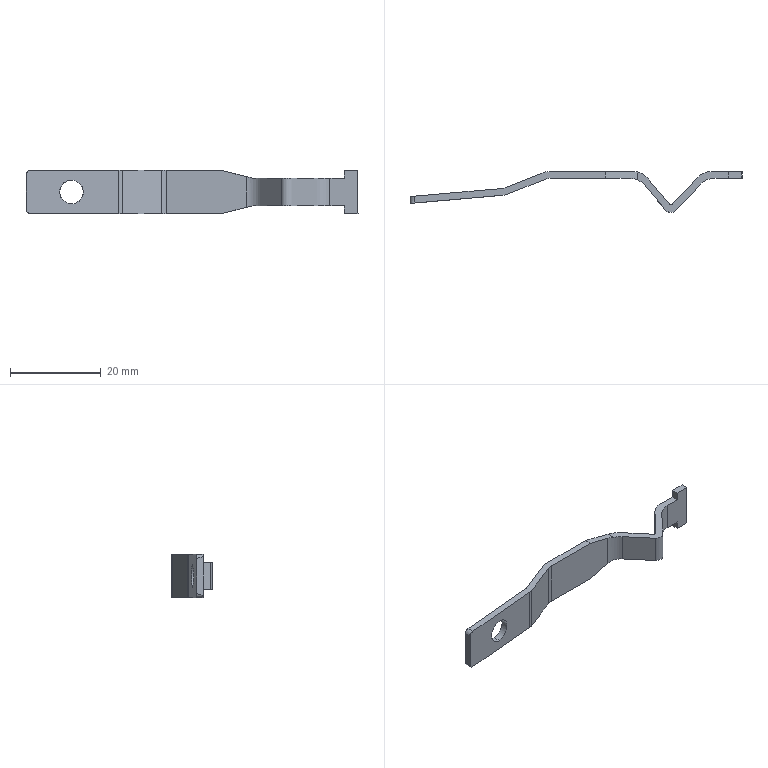Part | SolidWorks | features Extrusion 1, ICE 1 | 1 solid | 38 faces | box 73 x 9 x 9.5 mm | volume 954.396 mm3 | plane 24 | cylinder 14 | commonest cylinder face diameters 6 x4 8 x4 2 x2 5.2 x2 1 x1 3 x1
STEP:
#1=CARTESIAN_POINT('',(72.28,15.995,-2.6));
#2=VERTEX_POINT('',#1);
#3=CARTESIAN_POINT('',(72.28,15.995,2.6));
#4=VERTEX_POINT('',#3);
#5=CARTESIAN_POINT('',(72.28,15.995,-2.6));
#6=CARTESIAN_POINT('',(67.08,15.54,-2.6));
#7=CARTESIAN_POINT('',(67.08,15.54,2.6));
#8=CARTESIAN_POINT('',(72.28,15.995,2.6));
#9=(BOUNDED_CURVE()B_SPLINE_CURVE(3,(#5,#6,#7,#8),.UNSPECIFIED.,.F.,.T.)B_SPLINE_CURVE_WITH_KNOTS((4,4),(4.712,7.854),.UNSPECIFIED.)CURVE()GEOMETRIC_REPRESENTATION_ITEM()RATIONAL_B_SPLINE_CURVE((1.,0.3333,0.3333,1.))REPRESENTATION_ITEM(''));
#10=EDGE_CURVE('',#2,#4,#9,.T.);
#11=ORIENTED_EDGE('',*,*,#10,.T.);
#12=CARTESIAN_POINT('',(72.28,14.489,2.6));
#13=VERTEX_POINT('',#12);
#14=CARTESIAN_POINT('',(72.28,30.,2.6));
#15=DIRECTION('',(0.,-1.,0.));
#16=VECTOR('',#15,1000.);
#17=LINE('',#14,#16);
#18=EDGE_CURVE('',#4,#13,#17,.T.);
#19=ORIENTED_EDGE('',*,*,#18,.T.);
#20=CARTESIAN_POINT('',(72.28,14.489,-2.6));
#21=VERTEX_POINT('',#20);
#22=CARTESIAN_POINT('',(72.28,14.489,2.6));
#23=CARTESIAN_POINT('',(67.08,14.035,2.6));
#24=CARTESIAN_POINT('',(67.08,14.035,-2.6));
#25=CARTESIAN_POINT('',(72.28,14.489,-2.6));
#26=(BOUNDED_CURVE()B_SPLINE_CURVE(3,(#22,#23,#24,#25),.UNSPECIFIED.,.F.,.T.)B_SPLINE_CURVE_WITH_KNOTS((4,4),(4.712,7.854),.UNSPECIFIED.)CURVE()GEOMETRIC_REPRESENTATION_ITEM()RATIONAL_B_SPLINE_CURVE((1.,0.3333,0.3333,1.))REPRESENTATION_ITEM(''));
#27=EDGE_CURVE('',#13,#21,#26,.T.);
#28=ORIENTED_EDGE('',*,*,#27,.T.);
#29=CARTESIAN_POINT('',(72.28,30.,-2.6));
#30=DIRECTION('',(0.,-1.,0.));
#31=VECTOR('',#30,1000.);
#32=LINE('',#29,#31);
#33=EDGE_CURVE('',#2,#21,#32,.T.);
#34=ORIENTED_EDGE('',*,*,#33,.F.);
#35=EDGE_LOOP('',(#11,#19,#28,#34));
#36=FACE_OUTER_BOUND('',#35,.T.);
#37=CARTESIAN_POINT('',(72.28,30.,0.));
#38=DIRECTION('',(0.,-1.,0.));
#39=DIRECTION('',(0.,0.,-1.));
#40=AXIS2_PLACEMENT_3D('',#37,#38,#39);
#41=CYLINDRICAL_SURFACE('',#40,2.6);
#42=ADVANCED_FACE('',(#36),#41,.F.);
#43=CARTESIAN_POINT('',(63.28,13.702,4.75));
#44=VERTEX_POINT('',#43);
#45=CARTESIAN_POINT('',(63.28,15.208,4.75));
#46=VERTEX_POINT('',#45);
#47=CARTESIAN_POINT('',(63.28,30.,4.75));
#48=DIRECTION('',(0.,1.,0.));
#49=VECTOR('',#48,1000.);
#50=LINE('',#47,#49);
#51=EDGE_CURVE('',#44,#46,#50,.T.);
#52=ORIENTED_EDGE('',*,*,#51,.F.);
#53=CARTESIAN_POINT('',(82.696,15.401,4.75));
#54=VERTEX_POINT('',#53);
#55=CARTESIAN_POINT('',(62.41,13.626,4.75));
#56=DIRECTION('',(0.9962,0.08716,0.));
#57=VECTOR('',#56,1000.);
#58=LINE('',#55,#57);
#59=EDGE_CURVE('',#44,#54,#58,.T.);
#60=ORIENTED_EDGE('',*,*,#59,.T.);
#61=CARTESIAN_POINT('',(83.526,15.595,4.75));
#62=VERTEX_POINT('',#61);
#63=CARTESIAN_POINT('',(82.434,18.389,4.75));
#64=DIRECTION('',(0.,0.,1.));
#65=DIRECTION('',(1.,0.,0.));
#66=AXIS2_PLACEMENT_3D('',#63,#64,#65);
#67=CIRCLE('',#66,3.);
#68=EDGE_CURVE('',#54,#62,#67,.T.);
#69=ORIENTED_EDGE('',*,*,#68,.T.);
#70=CARTESIAN_POINT('',(92.036,18.92,4.75));
#71=VERTEX_POINT('',#70);
#72=CARTESIAN_POINT('',(83.526,15.595,4.75));
#73=DIRECTION('',(0.9314,0.364,0.));
#74=VECTOR('',#73,1000.);
#75=LINE('',#72,#74);
#76=EDGE_CURVE('',#62,#71,#75,.T.);
#77=ORIENTED_EDGE('',*,*,#76,.T.);
#78=CARTESIAN_POINT('',(93.127,19.126,4.75));
#79=VERTEX_POINT('',#78);
#80=CARTESIAN_POINT('',(93.127,16.126,4.75));
#81=DIRECTION('',(0.,0.,-1.));
#82=DIRECTION('',(1.,0.,0.));
#83=AXIS2_PLACEMENT_3D('',#80,#81,#82);
#84=CIRCLE('',#83,3.);
#85=EDGE_CURVE('',#71,#79,#84,.T.);
#86=ORIENTED_EDGE('',*,*,#85,.T.);
#87=CARTESIAN_POINT('',(105.257,19.126,4.75));
#88=VERTEX_POINT('',#87);
#89=CARTESIAN_POINT('',(93.127,19.126,4.75));
#90=DIRECTION('',(1.,0.,0.));
#91=VECTOR('',#90,1000.);
#92=LINE('',#89,#91);
#93=EDGE_CURVE('',#79,#88,#92,.T.);
#94=ORIENTED_EDGE('',*,*,#93,.T.);
#95=CARTESIAN_POINT('',(105.257,20.626,4.75));
#96=VERTEX_POINT('',#95);
#97=CARTESIAN_POINT('',(105.257,19.865,4.75));
#98=DIRECTION('',(0.,1.,0.));
#99=VECTOR('',#98,1000.);
#100=LINE('',#97,#99);
#101=EDGE_CURVE('',#88,#96,#100,.T.);
#102=ORIENTED_EDGE('',*,*,#101,.T.);
#103=CARTESIAN_POINT('',(92.845,20.626,4.75));
#104=VERTEX_POINT('',#103);
#105=CARTESIAN_POINT('',(92.845,20.626,4.75));
#106=DIRECTION('',(-1.,0.,0.));
#107=VECTOR('',#106,1000.);
#108=LINE('',#105,#107);
#109=EDGE_CURVE('',#96,#104,#108,.T.);
#110=ORIENTED_EDGE('',*,*,#109,.T.);
#111=CARTESIAN_POINT('',(91.753,20.42,4.75));
#112=VERTEX_POINT('',#111);
#113=CARTESIAN_POINT('',(92.845,17.626,4.75));
#114=DIRECTION('',(0.,0.,1.));
#115=DIRECTION('',(-1.,0.,0.));
#116=AXIS2_PLACEMENT_3D('',#113,#114,#115);
#117=CIRCLE('',#116,3.);
#118=EDGE_CURVE('',#104,#112,#117,.T.);
#119=ORIENTED_EDGE('',*,*,#118,.T.);
#120=CARTESIAN_POINT('',(83.181,17.071,4.75));
#121=VERTEX_POINT('',#120);
#122=CARTESIAN_POINT('',(83.181,17.071,4.75));
#123=DIRECTION('',(-0.9314,-0.364,0.));
#124=VECTOR('',#123,1000.);
#125=LINE('',#122,#124);
#126=EDGE_CURVE('',#112,#121,#125,.T.);
#127=ORIENTED_EDGE('',*,*,#126,.T.);
#128=CARTESIAN_POINT('',(82.35,16.876,4.75));
#129=VERTEX_POINT('',#128);
#130=CARTESIAN_POINT('',(82.089,19.865,4.75));
#131=DIRECTION('',(0.,0.,-1.));
#132=DIRECTION('',(-1.,0.,0.));
#133=AXIS2_PLACEMENT_3D('',#130,#131,#132);
#134=CIRCLE('',#133,3.);
#135=EDGE_CURVE('',#121,#129,#134,.T.);
#136=ORIENTED_EDGE('',*,*,#135,.T.);
#137=CARTESIAN_POINT('',(62.28,15.12,4.75));
#138=DIRECTION('',(-0.9962,-0.08716,0.));
#139=VECTOR('',#138,1000.);
#140=LINE('',#137,#139);
#141=EDGE_CURVE('',#129,#46,#140,.T.);
#142=ORIENTED_EDGE('',*,*,#141,.T.);
#143=EDGE_LOOP('',(#52,#60,#69,#77,#86,#94,#102,#110,#119,#127,#136,#142));
#144=FACE_OUTER_BOUND('',#143,.T.);
#145=CARTESIAN_POINT('',(82.089,19.865,4.75));
#146=DIRECTION('',(0.,0.,-1.));
#147=DIRECTION('',(-1.,0.,0.));
#148=AXIS2_PLACEMENT_3D('',#145,#146,#147);
#149=PLANE('',#148);
#150=ADVANCED_FACE('',(#144),#149,.F.);
#151=CARTESIAN_POINT('',(132.28,20.626,-4.75));
#152=VERTEX_POINT('',#151);
#153=CARTESIAN_POINT('',(132.28,19.126,-4.75));
#154=VERTEX_POINT('',#153);
#155=CARTESIAN_POINT('',(132.28,19.865,-4.75));
#156=DIRECTION('',(0.,-1.,0.));
#157=VECTOR('',#156,1000.);
#158=LINE('',#155,#157);
#159=EDGE_CURVE('',#152,#154,#158,.T.);
#160=ORIENTED_EDGE('',*,*,#159,.F.);
#161=CARTESIAN_POINT('',(135.28,20.626,-4.75));
#162=VERTEX_POINT('',#161);
#163=CARTESIAN_POINT('',(128.472,20.626,-4.75));
#164=DIRECTION('',(-1.,0.,0.));
#165=VECTOR('',#164,1000.);
#166=LINE('',#163,#165);
#167=EDGE_CURVE('',#162,#152,#166,.T.);
#168=ORIENTED_EDGE('',*,*,#167,.F.);
#169=CARTESIAN_POINT('',(135.28,19.126,-4.75));
#170=VERTEX_POINT('',#169);
#171=CARTESIAN_POINT('',(135.28,19.126,-4.75));
#172=DIRECTION('',(0.,1.,0.));
#173=VECTOR('',#172,1000.);
#174=LINE('',#171,#173);
#175=EDGE_CURVE('',#170,#162,#174,.T.);
#176=ORIENTED_EDGE('',*,*,#175,.F.);
#177=CARTESIAN_POINT('',(129.116,19.126,-4.75));
#178=DIRECTION('',(1.,0.,0.));
#179=VECTOR('',#178,1000.);
#180=LINE('',#177,#179);
#181=EDGE_CURVE('',#154,#170,#180,.T.);
#182=ORIENTED_EDGE('',*,*,#181,.F.);
#183=EDGE_LOOP('',(#160,#168,#176,#182));
#184=FACE_OUTER_BOUND('',#183,.T.);
#185=CARTESIAN_POINT('',(82.089,19.865,-4.75));
#186=DIRECTION('',(0.,0.,-1.));
#187=DIRECTION('',(-1.,0.,0.));
#188=AXIS2_PLACEMENT_3D('',#185,#186,#187);
#189=PLANE('',#188);
#190=ADVANCED_FACE('',(#184),#189,.T.);
#191=CARTESIAN_POINT('',(105.257,19.126,-4.75));
#192=VERTEX_POINT('',#191);
#193=CARTESIAN_POINT('',(105.257,20.626,-4.75));
#194=VERTEX_POINT('',#193);
#195=CARTESIAN_POINT('',(105.257,19.865,-4.75));
#196=DIRECTION('',(0.,1.,0.));
#197=VECTOR('',#196,1000.);
#198=LINE('',#195,#197);
#199=EDGE_CURVE('',#192,#194,#198,.T.);
#200=ORIENTED_EDGE('',*,*,#199,.F.);
#201=CARTESIAN_POINT('',(93.127,19.126,-4.75));
#202=VERTEX_POINT('',#201);
#203=CARTESIAN_POINT('',(93.127,19.126,-4.75));
#204=DIRECTION('',(1.,0.,0.));
#205=VECTOR('',#204,1000.);
#206=LINE('',#203,#205);
#207=EDGE_CURVE('',#202,#192,#206,.T.);
#208=ORIENTED_EDGE('',*,*,#207,.F.);
#209=CARTESIAN_POINT('',(92.036,18.92,-4.75));
#210=VERTEX_POINT('',#209);
#211=CARTESIAN_POINT('',(93.127,16.126,-4.75));
#212=DIRECTION('',(0.,0.,-1.));
#213=DIRECTION('',(1.,0.,0.));
#214=AXIS2_PLACEMENT_3D('',#211,#212,#213);
#215=CIRCLE('',#214,3.);
#216=EDGE_CURVE('',#210,#202,#215,.T.);
#217=ORIENTED_EDGE('',*,*,#216,.F.);
#218=CARTESIAN_POINT('',(83.526,15.595,-4.75));
#219=VERTEX_POINT('',#218);
#220=CARTESIAN_POINT('',(83.526,15.595,-4.75));
#221=DIRECTION('',(0.9314,0.364,0.));
#222=VECTOR('',#221,1000.);
#223=LINE('',#220,#222);
#224=EDGE_CURVE('',#219,#210,#223,.T.);
#225=ORIENTED_EDGE('',*,*,#224,.F.);
#226=CARTESIAN_POINT('',(82.696,15.401,-4.75));
#227=VERTEX_POINT('',#226);
#228=CARTESIAN_POINT('',(82.434,18.389,-4.75));
#229=DIRECTION('',(0.,0.,1.));
#230=DIRECTION('',(1.,0.,0.));
#231=AXIS2_PLACEMENT_3D('',#228,#229,#230);
#232=CIRCLE('',#231,3.);
#233=EDGE_CURVE('',#227,#219,#232,.T.);
#234=ORIENTED_EDGE('',*,*,#233,.F.);
#235=CARTESIAN_POINT('',(63.28,13.702,-4.75));
#236=VERTEX_POINT('',#235);
#237=CARTESIAN_POINT('',(62.41,13.626,-4.75));
#238=DIRECTION('',(0.9962,0.08716,0.));
#239=VECTOR('',#238,1000.);
#240=LINE('',#237,#239);
#241=EDGE_CURVE('',#236,#227,#240,.T.);
#242=ORIENTED_EDGE('',*,*,#241,.F.);
#243=CARTESIAN_POINT('',(63.28,15.208,-4.75));
#244=VERTEX_POINT('',#243);
#245=CARTESIAN_POINT('',(63.28,30.,-4.75));
#246=DIRECTION('',(0.,1.,0.));
#247=VECTOR('',#246,1000.);
#248=LINE('',#245,#247);
#249=EDGE_CURVE('',#236,#244,#248,.T.);
#250=ORIENTED_EDGE('',*,*,#249,.T.);
#251=CARTESIAN_POINT('',(82.35,16.876,-4.75));
#252=VERTEX_POINT('',#251);
#253=CARTESIAN_POINT('',(62.28,15.12,-4.75));
#254=DIRECTION('',(-0.9962,-0.08716,0.));
#255=VECTOR('',#254,1000.);
#256=LINE('',#253,#255);
#257=EDGE_CURVE('',#252,#244,#256,.T.);
#258=ORIENTED_EDGE('',*,*,#257,.F.);
#259=CARTESIAN_POINT('',(83.181,17.071,-4.75));
#260=VERTEX_POINT('',#259);
#261=CARTESIAN_POINT('',(82.089,19.865,-4.75));
#262=DIRECTION('',(0.,0.,-1.));
#263=DIRECTION('',(-1.,0.,0.));
#264=AXIS2_PLACEMENT_3D('',#261,#262,#263);
#265=CIRCLE('',#264,3.);
#266=EDGE_CURVE('',#260,#252,#265,.T.);
#267=ORIENTED_EDGE('',*,*,#266,.F.);
#268=CARTESIAN_POINT('',(91.753,20.42,-4.75));
#269=VERTEX_POINT('',#268);
#270=CARTESIAN_POINT('',(83.181,17.071,-4.75));
#271=DIRECTION('',(-0.9314,-0.364,0.));
#272=VECTOR('',#271,1000.);
#273=LINE('',#270,#272);
#274=EDGE_CURVE('',#269,#260,#273,.T.);
#275=ORIENTED_EDGE('',*,*,#274,.F.);
#276=CARTESIAN_POINT('',(92.845,20.626,-4.75));
#277=VERTEX_POINT('',#276);
#278=CARTESIAN_POINT('',(92.845,17.626,-4.75));
#279=DIRECTION('',(0.,0.,1.));
#280=DIRECTION('',(-1.,0.,0.));
#281=AXIS2_PLACEMENT_3D('',#278,#279,#280);
#282=CIRCLE('',#281,3.);
#283=EDGE_CURVE('',#277,#269,#282,.T.);
#284=ORIENTED_EDGE('',*,*,#283,.F.);
#285=CARTESIAN_POINT('',(92.845,20.626,-4.75));
#286=DIRECTION('',(-1.,0.,0.));
#287=VECTOR('',#286,1000.);
#288=LINE('',#285,#287);
#289=EDGE_CURVE('',#194,#277,#288,.T.);
#290=ORIENTED_EDGE('',*,*,#289,.F.);
#291=EDGE_LOOP('',(#200,#208,#217,#225,#234,#242,#250,#258,#267,#275,#284,#290));
#292=FACE_OUTER_BOUND('',#291,.T.);
#293=CARTESIAN_POINT('',(82.089,19.865,-4.75));
#294=DIRECTION('',(0.,0.,-1.));
#295=DIRECTION('',(-1.,0.,0.));
#296=AXIS2_PLACEMENT_3D('',#293,#294,#295);
#297=PLANE('',#296);
#298=ADVANCED_FACE('',(#292),#297,.T.);
#299=CARTESIAN_POINT('',(62.41,13.626,4.244));
#300=VERTEX_POINT('',#299);
#301=CARTESIAN_POINT('',(62.41,13.626,-4.244));
#302=VERTEX_POINT('',#301);
#303=CARTESIAN_POINT('',(62.41,13.626,4.75));
#304=DIRECTION('',(0.,0.,-1.));
#305=VECTOR('',#304,1000.);
#306=LINE('',#303,#305);
#307=EDGE_CURVE('',#300,#302,#306,.T.);
#308=ORIENTED_EDGE('',*,*,#307,.T.);
#309=CARTESIAN_POINT('',(62.41,13.626,-4.244));
#310=CARTESIAN_POINT('',(62.592,13.642,-4.565));
#311=CARTESIAN_POINT('',(62.911,13.67,-4.75));
#312=CARTESIAN_POINT('',(63.28,13.702,-4.75));
#313=(BOUNDED_CURVE()B_SPLINE_CURVE(3,(#309,#310,#311,#312),.UNSPECIFIED.,.F.,.T.)B_SPLINE_CURVE_WITH_KNOTS((4,4),(0.5171,1.571),.UNSPECIFIED.)CURVE()GEOMETRIC_REPRESENTATION_ITEM()RATIONAL_B_SPLINE_CURVE((1.,0.9096,0.9096,1.))REPRESENTATION_ITEM(''));
#314=EDGE_CURVE('',#302,#236,#313,.T.);
#315=ORIENTED_EDGE('',*,*,#314,.T.);
#316=ORIENTED_EDGE('',*,*,#241,.T.);
#317=CARTESIAN_POINT('',(82.696,15.401,4.75));
#318=DIRECTION('',(0.,0.,-1.));
#319=VECTOR('',#318,1000.);
#320=LINE('',#317,#319);
#321=EDGE_CURVE('',#54,#227,#320,.T.);
#322=ORIENTED_EDGE('',*,*,#321,.F.);
#323=ORIENTED_EDGE('',*,*,#59,.F.);
#324=CARTESIAN_POINT('',(63.28,13.702,4.75));
#325=CARTESIAN_POINT('',(62.911,13.67,4.75));
#326=CARTESIAN_POINT('',(62.592,13.642,4.565));
#327=CARTESIAN_POINT('',(62.41,13.626,4.244));
#328=(BOUNDED_CURVE()B_SPLINE_CURVE(3,(#324,#325,#326,#327),.UNSPECIFIED.,.F.,.T.)B_SPLINE_CURVE_WITH_KNOTS((4,4),(4.712,5.766),.UNSPECIFIED.)CURVE()GEOMETRIC_REPRESENTATION_ITEM()RATIONAL_B_SPLINE_CURVE((1.,0.9096,0.9096,1.))REPRESENTATION_ITEM(''));
#329=EDGE_CURVE('',#44,#300,#328,.T.);
#330=ORIENTED_EDGE('',*,*,#329,.T.);
#331=EDGE_LOOP('',(#308,#315,#316,#322,#323,#330));
#332=FACE_OUTER_BOUND('',#331,.T.);
#333=CARTESIAN_POINT('',(72.28,14.489,-2.6));
#334=CARTESIAN_POINT('',(77.48,14.944,-2.6));
#335=CARTESIAN_POINT('',(77.48,14.944,2.6));
#336=CARTESIAN_POINT('',(72.28,14.489,2.6));
#337=(BOUNDED_CURVE()B_SPLINE_CURVE(3,(#333,#334,#335,#336),.UNSPECIFIED.,.F.,.T.)B_SPLINE_CURVE_WITH_KNOTS((4,4),(1.571,4.712),.UNSPECIFIED.)CURVE()GEOMETRIC_REPRESENTATION_ITEM()RATIONAL_B_SPLINE_CURVE((1.,0.3333,0.3333,1.))REPRESENTATION_ITEM(''));
#338=EDGE_CURVE('',#21,#13,#337,.T.);
#339=ORIENTED_EDGE('',*,*,#338,.F.);
#340=ORIENTED_EDGE('',*,*,#27,.F.);
#341=EDGE_LOOP('',(#339,#340));
#342=FACE_BOUND('',#341,.T.);
#343=CARTESIAN_POINT('',(62.41,13.626,4.75));
#344=DIRECTION('',(-0.08716,0.9962,0.));
#345=DIRECTION('',(-0.9962,-0.08716,0.));
#346=AXIS2_PLACEMENT_3D('',#343,#344,#345);
#347=PLANE('',#346);
#348=ADVANCED_FACE('',(#332,#342),#347,.F.);
#349=ORIENTED_EDGE('',*,*,#257,.T.);
#350=CARTESIAN_POINT('',(62.28,15.12,-3.75));
#351=VERTEX_POINT('',#350);
#352=CARTESIAN_POINT('',(63.28,15.208,-4.75));
#353=CARTESIAN_POINT('',(62.694,15.157,-4.75));
#354=CARTESIAN_POINT('',(62.28,15.12,-4.336));
#355=CARTESIAN_POINT('',(62.28,15.12,-3.75));
#356=(BOUNDED_CURVE()B_SPLINE_CURVE(3,(#352,#353,#354,#355),.UNSPECIFIED.,.F.,.T.)B_SPLINE_CURVE_WITH_KNOTS((4,4),(4.712,6.283),.UNSPECIFIED.)CURVE()GEOMETRIC_REPRESENTATION_ITEM()RATIONAL_B_SPLINE_CURVE((1.,0.8047,0.8047,1.))REPRESENTATION_ITEM(''));
#357=EDGE_CURVE('',#244,#351,#356,.T.);
#358=ORIENTED_EDGE('',*,*,#357,.T.);
#359=CARTESIAN_POINT('',(62.28,15.12,3.75));
#360=VERTEX_POINT('',#359);
#361=CARTESIAN_POINT('',(62.28,15.12,4.75));
#362=DIRECTION('',(0.,0.,-1.));
#363=VECTOR('',#362,1000.);
#364=LINE('',#361,#363);
#365=EDGE_CURVE('',#360,#351,#364,.T.);
#366=ORIENTED_EDGE('',*,*,#365,.F.);
#367=CARTESIAN_POINT('',(62.28,15.12,3.75));
#368=CARTESIAN_POINT('',(62.28,15.12,4.336));
#369=CARTESIAN_POINT('',(62.694,15.157,4.75));
#370=CARTESIAN_POINT('',(63.28,15.208,4.75));
#371=(BOUNDED_CURVE()B_SPLINE_CURVE(3,(#367,#368,#369,#370),.UNSPECIFIED.,.F.,.F.)B_SPLINE_CURVE_WITH_KNOTS((4,4),(0.,1.571),.UNSPECIFIED.)CURVE()GEOMETRIC_REPRESENTATION_ITEM()RATIONAL_B_SPLINE_CURVE((1.,0.8047,0.8047,1.))REPRESENTATION_ITEM(''));
#372=EDGE_CURVE('',#360,#46,#371,.T.);
#373=ORIENTED_EDGE('',*,*,#372,.T.);
#374=ORIENTED_EDGE('',*,*,#141,.F.);
#375=CARTESIAN_POINT('',(82.35,16.876,4.75));
#376=DIRECTION('',(0.,0.,-1.));
#377=VECTOR('',#376,1000.);
#378=LINE('',#375,#377);
#379=EDGE_CURVE('',#129,#252,#378,.T.);
#380=ORIENTED_EDGE('',*,*,#379,.T.);
#381=EDGE_LOOP('',(#349,#358,#366,#373,#374,#380));
#382=FACE_OUTER_BOUND('',#381,.T.);
#383=ORIENTED_EDGE('',*,*,#10,.F.);
#384=CARTESIAN_POINT('',(72.28,15.995,2.6));
#385=CARTESIAN_POINT('',(77.48,16.45,2.6));
#386=CARTESIAN_POINT('',(77.48,16.45,-2.6));
#387=CARTESIAN_POINT('',(72.28,15.995,-2.6));
#388=(BOUNDED_CURVE()B_SPLINE_CURVE(3,(#384,#385,#386,#387),.UNSPECIFIED.,.F.,.T.)B_SPLINE_CURVE_WITH_KNOTS((4,4),(1.571,4.712),.UNSPECIFIED.)CURVE()GEOMETRIC_REPRESENTATION_ITEM()RATIONAL_B_SPLINE_CURVE((1.,0.3333,0.3333,1.))REPRESENTATION_ITEM(''));
#389=EDGE_CURVE('',#4,#2,#388,.T.);
#390=ORIENTED_EDGE('',*,*,#389,.F.);
#391=EDGE_LOOP('',(#383,#390));
#392=FACE_BOUND('',#391,.T.);
#393=CARTESIAN_POINT('',(62.28,15.12,4.75));
#394=DIRECTION('',(0.08716,-0.9962,0.));
#395=DIRECTION('',(0.9962,0.08716,0.));
#396=AXIS2_PLACEMENT_3D('',#393,#394,#395);
#397=PLANE('',#396);
#398=ADVANCED_FACE('',(#382,#392),#397,.F.);
#399=ORIENTED_EDGE('',*,*,#365,.T.);
#400=CARTESIAN_POINT('',(62.28,15.12,-3.75));
#401=CARTESIAN_POINT('',(62.28,15.12,-3.924));
#402=CARTESIAN_POINT('',(62.324,14.611,-4.093));
#403=CARTESIAN_POINT('',(62.41,13.626,-4.244));
#404=(BOUNDED_CURVE()B_SPLINE_CURVE(3,(#400,#401,#402,#403),.UNSPECIFIED.,.F.,.T.)B_SPLINE_CURVE_WITH_KNOTS((4,4),(3.142,3.659),.UNSPECIFIED.)CURVE()GEOMETRIC_REPRESENTATION_ITEM()RATIONAL_B_SPLINE_CURVE((1.,0.9778,0.9778,1.))REPRESENTATION_ITEM(''));
#405=EDGE_CURVE('',#351,#302,#404,.T.);
#406=ORIENTED_EDGE('',*,*,#405,.T.);
#407=ORIENTED_EDGE('',*,*,#307,.F.);
#408=CARTESIAN_POINT('',(62.41,13.626,4.244));
#409=CARTESIAN_POINT('',(62.324,14.611,4.093));
#410=CARTESIAN_POINT('',(62.28,15.12,3.924));
#411=CARTESIAN_POINT('',(62.28,15.12,3.75));
#412=(BOUNDED_CURVE()B_SPLINE_CURVE(3,(#408,#409,#410,#411),.UNSPECIFIED.,.F.,.T.)B_SPLINE_CURVE_WITH_KNOTS((4,4),(2.625,3.142),.UNSPECIFIED.)CURVE()GEOMETRIC_REPRESENTATION_ITEM()RATIONAL_B_SPLINE_CURVE((1.,0.9778,0.9778,1.))REPRESENTATION_ITEM(''));
#413=EDGE_CURVE('',#300,#360,#412,.T.);
#414=ORIENTED_EDGE('',*,*,#413,.T.);
#415=EDGE_LOOP('',(#399,#406,#407,#414));
#416=FACE_OUTER_BOUND('',#415,.T.);
#417=CARTESIAN_POINT('',(62.41,13.626,4.75));
#418=DIRECTION('',(0.9962,0.08716,0.));
#419=DIRECTION('',(-0.08716,0.9962,0.));
#420=AXIS2_PLACEMENT_3D('',#417,#418,#419);
#421=PLANE('',#420);
#422=ADVANCED_FACE('',(#416),#421,.F.);
#423=ORIENTED_EDGE('',*,*,#233,.T.);
#424=CARTESIAN_POINT('',(83.526,15.595,4.75));
#425=DIRECTION('',(0.,0.,-1.));
#426=VECTOR('',#425,1000.);
#427=LINE('',#424,#426);
#428=EDGE_CURVE('',#62,#219,#427,.T.);
#429=ORIENTED_EDGE('',*,*,#428,.F.);
#430=ORIENTED_EDGE('',*,*,#68,.F.);
#431=ORIENTED_EDGE('',*,*,#321,.T.);
#432=EDGE_LOOP('',(#423,#429,#430,#431));
#433=FACE_OUTER_BOUND('',#432,.T.);
#434=CARTESIAN_POINT('',(82.434,18.389,4.75));
#435=DIRECTION('',(0.,0.,-1.));
#436=DIRECTION('',(-1.,0.,0.));
#437=AXIS2_PLACEMENT_3D('',#434,#435,#436);
#438=CYLINDRICAL_SURFACE('',#437,3.);
#439=ADVANCED_FACE('',(#433),#438,.T.);
#440=ORIENTED_EDGE('',*,*,#224,.T.);
#441=CARTESIAN_POINT('',(92.036,18.92,4.75));
#442=DIRECTION('',(0.,0.,-1.));
#443=VECTOR('',#442,1000.);
#444=LINE('',#441,#443);
#445=EDGE_CURVE('',#71,#210,#444,.T.);
#446=ORIENTED_EDGE('',*,*,#445,.F.);
#447=ORIENTED_EDGE('',*,*,#76,.F.);
#448=ORIENTED_EDGE('',*,*,#428,.T.);
#449=EDGE_LOOP('',(#440,#446,#447,#448));
#450=FACE_OUTER_BOUND('',#449,.T.);
#451=CARTESIAN_POINT('',(83.526,15.595,4.75));
#452=DIRECTION('',(-0.364,0.9314,0.));
#453=DIRECTION('',(-0.9314,-0.364,0.));
#454=AXIS2_PLACEMENT_3D('',#451,#452,#453);
#455=PLANE('',#454);
#456=ADVANCED_FACE('',(#450),#455,.F.);
#457=ORIENTED_EDGE('',*,*,#216,.T.);
#458=CARTESIAN_POINT('',(93.127,19.126,4.75));
#459=DIRECTION('',(0.,0.,-1.));
#460=VECTOR('',#459,1000.);
#461=LINE('',#458,#460);
#462=EDGE_CURVE('',#79,#202,#461,.T.);
#463=ORIENTED_EDGE('',*,*,#462,.F.);
#464=ORIENTED_EDGE('',*,*,#85,.F.);
#465=ORIENTED_EDGE('',*,*,#445,.T.);
#466=EDGE_LOOP('',(#457,#463,#464,#465));
#467=FACE_OUTER_BOUND('',#466,.T.);
#468=CARTESIAN_POINT('',(93.127,16.126,4.75));
#469=DIRECTION('',(0.,0.,-1.));
#470=DIRECTION('',(-1.,0.,0.));
#471=AXIS2_PLACEMENT_3D('',#468,#469,#470);
#472=CYLINDRICAL_SURFACE('',#471,3.);
#473=ADVANCED_FACE('',(#467),#472,.F.);
#474=ORIENTED_EDGE('',*,*,#207,.T.);
#475=CARTESIAN_POINT('',(110.731,19.126,-3.381));
#476=VERTEX_POINT('',#475);
#477=CARTESIAN_POINT('',(96.076,19.126,-7.045));
#478=DIRECTION('',(0.9701,0.,0.2425));
#479=VECTOR('',#478,1000.);
#480=LINE('',#477,#479);
#481=EDGE_CURVE('',#192,#476,#480,.T.);
#482=ORIENTED_EDGE('',*,*,#481,.T.);
#483=CARTESIAN_POINT('',(110.731,19.126,3.381));
#484=VERTEX_POINT('',#483);
#485=CARTESIAN_POINT('',(110.731,19.126,4.75));
#486=DIRECTION('',(0.,0.,-1.));
#487=VECTOR('',#486,1000.);
#488=LINE('',#485,#487);
#489=EDGE_CURVE('',#484,#476,#488,.T.);
#490=ORIENTED_EDGE('',*,*,#489,.F.);
#491=CARTESIAN_POINT('',(93.841,19.126,7.604));
#492=DIRECTION('',(-0.9701,0.,0.2425));
#493=VECTOR('',#492,1000.);
#494=LINE('',#491,#493);
#495=EDGE_CURVE('',#484,#88,#494,.T.);
#496=ORIENTED_EDGE('',*,*,#495,.T.);
#497=ORIENTED_EDGE('',*,*,#93,.F.);
#498=ORIENTED_EDGE('',*,*,#462,.T.);
#499=EDGE_LOOP('',(#474,#482,#490,#496,#497,#498));
#500=FACE_OUTER_BOUND('',#499,.T.);
#501=CARTESIAN_POINT('',(93.127,19.126,4.75));
#502=DIRECTION('',(0.,1.,0.));
#503=DIRECTION('',(-1.,0.,0.));
#504=AXIS2_PLACEMENT_3D('',#501,#502,#503);
#505=PLANE('',#504);
#506=ADVANCED_FACE('',(#500),#505,.F.);
#507=CARTESIAN_POINT('',(112.257,18.824,-3.));
#508=VERTEX_POINT('',#507);
#509=CARTESIAN_POINT('',(110.731,19.126,-3.381));
#510=CARTESIAN_POINT('',(111.256,19.126,-3.25));
#511=CARTESIAN_POINT('',(111.771,19.024,-3.121));
#512=CARTESIAN_POINT('',(112.257,18.824,-3.));
#513=(BOUNDED_CURVE()B_SPLINE_CURVE(3,(#509,#510,#511,#512),.UNSPECIFIED.,.F.,.T.)B_SPLINE_CURVE_WITH_KNOTS((4,4),(1.571,1.962),.UNSPECIFIED.)CURVE()GEOMETRIC_REPRESENTATION_ITEM()RATIONAL_B_SPLINE_CURVE((1.,0.9873,0.9873,1.))REPRESENTATION_ITEM(''));
#514=EDGE_CURVE('',#476,#508,#513,.T.);
#515=ORIENTED_EDGE('',*,*,#514,.T.);
#516=CARTESIAN_POINT('',(113.783,17.712,-3.));
#517=VERTEX_POINT('',#516);
#518=CARTESIAN_POINT('',(110.731,15.126,-3.));
#519=DIRECTION('',(0.,0.,-1.));
#520=DIRECTION('',(1.,0.,0.));
#521=AXIS2_PLACEMENT_3D('',#518,#519,#520);
#522=CIRCLE('',#521,4.);
#523=EDGE_CURVE('',#508,#517,#522,.T.);
#524=ORIENTED_EDGE('',*,*,#523,.T.);
#525=CARTESIAN_POINT('',(113.783,17.712,3.));
#526=VERTEX_POINT('',#525);
#527=CARTESIAN_POINT('',(113.783,17.712,4.75));
#528=DIRECTION('',(0.,0.,-1.));
#529=VECTOR('',#528,1000.);
#530=LINE('',#527,#529);
#531=EDGE_CURVE('',#526,#517,#530,.T.);
#532=ORIENTED_EDGE('',*,*,#531,.F.);
#533=CARTESIAN_POINT('',(112.257,18.824,3.));
#534=VERTEX_POINT('',#533);
#535=CARTESIAN_POINT('',(110.731,15.126,3.));
#536=DIRECTION('',(0.,0.,1.));
#537=DIRECTION('',(-1.,0.,0.));
#538=AXIS2_PLACEMENT_3D('',#535,#536,#537);
#539=CIRCLE('',#538,4.);
#540=EDGE_CURVE('',#526,#534,#539,.T.);
#541=ORIENTED_EDGE('',*,*,#540,.T.);
#542=CARTESIAN_POINT('',(112.257,18.824,3.));
#543=CARTESIAN_POINT('',(111.771,19.024,3.121));
#544=CARTESIAN_POINT('',(111.256,19.126,3.25));
#545=CARTESIAN_POINT('',(110.731,19.126,3.381));
#546=(BOUNDED_CURVE()B_SPLINE_CURVE(3,(#542,#543,#544,#545),.UNSPECIFIED.,.F.,.T.)B_SPLINE_CURVE_WITH_KNOTS((4,4),(1.179,1.571),.UNSPECIFIED.)CURVE()GEOMETRIC_REPRESENTATION_ITEM()RATIONAL_B_SPLINE_CURVE((1.,0.9873,0.9873,1.))REPRESENTATION_ITEM(''));
#547=EDGE_CURVE('',#534,#484,#546,.T.);
#548=ORIENTED_EDGE('',*,*,#547,.T.);
#549=ORIENTED_EDGE('',*,*,#489,.T.);
#550=EDGE_LOOP('',(#515,#524,#532,#541,#548,#549));
#551=FACE_OUTER_BOUND('',#550,.T.);
#552=CARTESIAN_POINT('',(110.731,15.126,4.75));
#553=DIRECTION('',(0.,0.,-1.));
#554=DIRECTION('',(-1.,0.,0.));
#555=AXIS2_PLACEMENT_3D('',#552,#553,#554);
#556=CYLINDRICAL_SURFACE('',#555,4.);
#557=ADVANCED_FACE('',(#551),#556,.F.);
#558=ORIENTED_EDGE('',*,*,#531,.T.);
#559=CARTESIAN_POINT('',(118.491,12.156,-3.));
#560=VERTEX_POINT('',#559);
#561=CARTESIAN_POINT('',(113.783,17.712,-3.));
#562=DIRECTION('',(0.6465,-0.7629,0.));
#563=VECTOR('',#562,1000.);
#564=LINE('',#561,#563);
#565=EDGE_CURVE('',#517,#560,#564,.T.);
#566=ORIENTED_EDGE('',*,*,#565,.T.);
#567=CARTESIAN_POINT('',(118.491,12.156,3.));
#568=VERTEX_POINT('',#567);
#569=CARTESIAN_POINT('',(118.491,12.156,4.75));
#570=DIRECTION('',(0.,0.,-1.));
#571=VECTOR('',#570,1000.);
#572=LINE('',#569,#571);
#573=EDGE_CURVE('',#568,#560,#572,.T.);
#574=ORIENTED_EDGE('',*,*,#573,.F.);
#575=CARTESIAN_POINT('',(113.783,17.712,3.));
#576=DIRECTION('',(-0.6465,0.7629,0.));
#577=VECTOR('',#576,1000.);
#578=LINE('',#575,#577);
#579=EDGE_CURVE('',#568,#526,#578,.T.);
#580=ORIENTED_EDGE('',*,*,#579,.T.);
#581=EDGE_LOOP('',(#558,#566,#574,#580));
#582=FACE_OUTER_BOUND('',#581,.T.);
#583=CARTESIAN_POINT('',(113.783,17.712,4.75));
#584=DIRECTION('',(0.7629,0.6465,0.));
#585=DIRECTION('',(-0.6465,0.7629,0.));
#586=AXIS2_PLACEMENT_3D('',#583,#584,#585);
#587=PLANE('',#586);
#588=ADVANCED_FACE('',(#582),#587,.F.);
#589=ORIENTED_EDGE('',*,*,#573,.T.);
#590=CARTESIAN_POINT('',(120.723,12.093,-3.));
#591=VERTEX_POINT('',#590);
#592=CARTESIAN_POINT('',(119.635,13.126,-3.));
#593=DIRECTION('',(0.,0.,1.));
#594=DIRECTION('',(1.,0.,0.));
#595=AXIS2_PLACEMENT_3D('',#592,#593,#594);
#596=CIRCLE('',#595,1.5);
#597=EDGE_CURVE('',#560,#591,#596,.T.);
#598=ORIENTED_EDGE('',*,*,#597,.T.);
#599=CARTESIAN_POINT('',(120.723,12.093,3.));
#600=VERTEX_POINT('',#599);
#601=CARTESIAN_POINT('',(120.723,12.093,4.75));
#602=DIRECTION('',(0.,0.,-1.));
#603=VECTOR('',#602,1000.);
#604=LINE('',#601,#603);
#605=EDGE_CURVE('',#600,#591,#604,.T.);
#606=ORIENTED_EDGE('',*,*,#605,.F.);
#607=CARTESIAN_POINT('',(119.635,13.126,3.));
#608=DIRECTION('',(0.,0.,-1.));
#609=DIRECTION('',(-1.,0.,0.));
#610=AXIS2_PLACEMENT_3D('',#607,#608,#609);
#611=CIRCLE('',#610,1.5);
#612=EDGE_CURVE('',#600,#568,#611,.T.);
#613=ORIENTED_EDGE('',*,*,#612,.T.);
#614=EDGE_LOOP('',(#589,#598,#606,#613));
#615=FACE_OUTER_BOUND('',#614,.T.);
#616=CARTESIAN_POINT('',(119.635,13.126,4.75));
#617=DIRECTION('',(0.,0.,-1.));
#618=DIRECTION('',(-1.,0.,0.));
#619=AXIS2_PLACEMENT_3D('',#616,#617,#618);
#620=CYLINDRICAL_SURFACE('',#619,1.5);
#621=ADVANCED_FACE('',(#615),#620,.T.);
#622=ORIENTED_EDGE('',*,*,#605,.T.);
#623=CARTESIAN_POINT('',(126.215,17.88,-3.));
#624=VERTEX_POINT('',#623);
#625=CARTESIAN_POINT('',(120.723,12.093,-3.));
#626=DIRECTION('',(0.6884,0.7253,0.));
#627=VECTOR('',#626,1000.);
#628=LINE('',#625,#627);
#629=EDGE_CURVE('',#591,#624,#628,.T.);
#630=ORIENTED_EDGE('',*,*,#629,.T.);
#631=CARTESIAN_POINT('',(126.215,17.88,3.));
#632=VERTEX_POINT('',#631);
#633=CARTESIAN_POINT('',(126.215,17.88,4.75));
#634=DIRECTION('',(0.,0.,-1.));
#635=VECTOR('',#634,1000.);
#636=LINE('',#633,#635);
#637=EDGE_CURVE('',#632,#624,#636,.T.);
#638=ORIENTED_EDGE('',*,*,#637,.F.);
#639=CARTESIAN_POINT('',(120.723,12.093,3.));
#640=DIRECTION('',(-0.6884,-0.7253,0.));
#641=VECTOR('',#640,1000.);
#642=LINE('',#639,#641);
#643=EDGE_CURVE('',#632,#600,#642,.T.);
#644=ORIENTED_EDGE('',*,*,#643,.T.);
#645=EDGE_LOOP('',(#622,#630,#638,#644));
#646=FACE_OUTER_BOUND('',#645,.T.);
#647=CARTESIAN_POINT('',(120.723,12.093,4.75));
#648=DIRECTION('',(-0.7253,0.6884,0.));
#649=DIRECTION('',(-0.6884,-0.7253,0.));
#650=AXIS2_PLACEMENT_3D('',#647,#648,#649);
#651=PLANE('',#650);
#652=ADVANCED_FACE('',(#646),#651,.F.);
#653=ORIENTED_EDGE('',*,*,#637,.T.);
#654=CARTESIAN_POINT('',(129.116,19.126,-3.));
#655=VERTEX_POINT('',#654);
#656=CARTESIAN_POINT('',(129.116,15.126,-3.));
#657=DIRECTION('',(0.,0.,-1.));
#658=DIRECTION('',(1.,0.,0.));
#659=AXIS2_PLACEMENT_3D('',#656,#657,#658);
#660=CIRCLE('',#659,4.);
#661=EDGE_CURVE('',#624,#655,#660,.T.);
#662=ORIENTED_EDGE('',*,*,#661,.T.);
#663=CARTESIAN_POINT('',(129.116,19.126,3.));
#664=VERTEX_POINT('',#663);
#665=CARTESIAN_POINT('',(129.116,19.126,4.75));
#666=DIRECTION('',(0.,0.,-1.));
#667=VECTOR('',#666,1000.);
#668=LINE('',#665,#667);
#669=EDGE_CURVE('',#664,#655,#668,.T.);
#670=ORIENTED_EDGE('',*,*,#669,.F.);
#671=CARTESIAN_POINT('',(129.116,15.126,3.));
#672=DIRECTION('',(0.,0.,1.));
#673=DIRECTION('',(-1.,0.,0.));
#674=AXIS2_PLACEMENT_3D('',#671,#672,#673);
#675=CIRCLE('',#674,4.);
#676=EDGE_CURVE('',#664,#632,#675,.T.);
#677=ORIENTED_EDGE('',*,*,#676,.T.);
#678=EDGE_LOOP('',(#653,#662,#670,#677));
#679=FACE_OUTER_BOUND('',#678,.T.);
#680=CARTESIAN_POINT('',(129.116,15.126,4.75));
#681=DIRECTION('',(0.,0.,-1.));
#682=DIRECTION('',(-1.,0.,0.));
#683=AXIS2_PLACEMENT_3D('',#680,#681,#682);
#684=CYLINDRICAL_SURFACE('',#683,4.);
#685=ADVANCED_FACE('',(#679),#684,.F.);
#686=CARTESIAN_POINT('',(132.28,19.126,-3.));
#687=VERTEX_POINT('',#686);
#688=CARTESIAN_POINT('',(129.116,19.126,-3.));
#689=DIRECTION('',(1.,0.,0.));
#690=VECTOR('',#689,1000.);
#691=LINE('',#688,#690);
#692=EDGE_CURVE('',#655,#687,#691,.T.);
#693=ORIENTED_EDGE('',*,*,#692,.T.);
#694=CARTESIAN_POINT('',(132.28,19.126,4.75));
#695=DIRECTION('',(0.,0.,-1.));
#696=VECTOR('',#695,1000.);
#697=LINE('',#694,#696);
#698=EDGE_CURVE('',#687,#154,#697,.T.);
#699=ORIENTED_EDGE('',*,*,#698,.T.);
#700=ORIENTED_EDGE('',*,*,#181,.T.);
#701=CARTESIAN_POINT('',(135.28,19.126,4.75));
#702=VERTEX_POINT('',#701);
#703=CARTESIAN_POINT('',(135.28,19.126,4.75));
#704=DIRECTION('',(0.,0.,-1.));
#705=VECTOR('',#704,1000.);
#706=LINE('',#703,#705);
#707=EDGE_CURVE('',#702,#170,#706,.T.);
#708=ORIENTED_EDGE('',*,*,#707,.F.);
#709=CARTESIAN_POINT('',(132.28,19.126,4.75));
#710=VERTEX_POINT('',#709);
#711=CARTESIAN_POINT('',(129.116,19.126,4.75));
#712=DIRECTION('',(1.,0.,0.));
#713=VECTOR('',#712,1000.);
#714=LINE('',#711,#713);
#715=EDGE_CURVE('',#710,#702,#714,.T.);
#716=ORIENTED_EDGE('',*,*,#715,.F.);
#717=CARTESIAN_POINT('',(132.28,19.126,3.));
#718=VERTEX_POINT('',#717);
#719=CARTESIAN_POINT('',(132.28,19.126,4.75));
#720=DIRECTION('',(0.,0.,-1.));
#721=VECTOR('',#720,1000.);
#722=LINE('',#719,#721);
#723=EDGE_CURVE('',#710,#718,#722,.T.);
#724=ORIENTED_EDGE('',*,*,#723,.T.);
#725=CARTESIAN_POINT('',(129.116,19.126,3.));
#726=DIRECTION('',(-1.,0.,0.));
#727=VECTOR('',#726,1000.);
#728=LINE('',#725,#727);
#729=EDGE_CURVE('',#718,#664,#728,.T.);
#730=ORIENTED_EDGE('',*,*,#729,.T.);
#731=ORIENTED_EDGE('',*,*,#669,.T.);
#732=EDGE_LOOP('',(#693,#699,#700,#708,#716,#724,#730,#731));
#733=FACE_OUTER_BOUND('',#732,.T.);
#734=CARTESIAN_POINT('',(129.116,19.126,4.75));
#735=DIRECTION('',(0.,1.,0.));
#736=DIRECTION('',(0.,0.,1.));
#737=AXIS2_PLACEMENT_3D('',#734,#735,#736);
#738=PLANE('',#737);
#739=ADVANCED_FACE('',(#733),#738,.F.);
#740=ORIENTED_EDGE('',*,*,#175,.T.);
#741=CARTESIAN_POINT('',(135.28,20.626,4.75));
#742=VERTEX_POINT('',#741);
#743=CARTESIAN_POINT('',(135.28,20.626,4.75));
#744=DIRECTION('',(0.,0.,-1.));
#745=VECTOR('',#744,1000.);
#746=LINE('',#743,#745);
#747=EDGE_CURVE('',#742,#162,#746,.T.);
#748=ORIENTED_EDGE('',*,*,#747,.F.);
#749=CARTESIAN_POINT('',(135.28,19.126,4.75));
#750=DIRECTION('',(0.,1.,0.));
#751=VECTOR('',#750,1000.);
#752=LINE('',#749,#751);
#753=EDGE_CURVE('',#702,#742,#752,.T.);
#754=ORIENTED_EDGE('',*,*,#753,.F.);
#755=ORIENTED_EDGE('',*,*,#707,.T.);
#756=EDGE_LOOP('',(#740,#748,#754,#755));
#757=FACE_OUTER_BOUND('',#756,.T.);
#758=CARTESIAN_POINT('',(135.28,19.126,4.75));
#759=DIRECTION('',(-1.,0.,0.));
#760=DIRECTION('',(0.,0.,1.));
#761=AXIS2_PLACEMENT_3D('',#758,#759,#760);
#762=PLANE('',#761);
#763=ADVANCED_FACE('',(#757),#762,.F.);
#764=ORIENTED_EDGE('',*,*,#167,.T.);
#765=CARTESIAN_POINT('',(132.28,20.626,-3.));
#766=VERTEX_POINT('',#765);
#767=CARTESIAN_POINT('',(132.28,20.626,4.75));
#768=DIRECTION('',(0.,0.,1.));
#769=VECTOR('',#768,1000.);
#770=LINE('',#767,#769);
#771=EDGE_CURVE('',#152,#766,#770,.T.);
#772=ORIENTED_EDGE('',*,*,#771,.T.);
#773=CARTESIAN_POINT('',(128.472,20.626,-3.));
#774=VERTEX_POINT('',#773);
#775=CARTESIAN_POINT('',(128.472,20.626,-3.));
#776=DIRECTION('',(-1.,0.,0.));
#777=VECTOR('',#776,1000.);
#778=LINE('',#775,#777);
#779=EDGE_CURVE('',#766,#774,#778,.T.);
#780=ORIENTED_EDGE('',*,*,#779,.T.);
#781=CARTESIAN_POINT('',(128.472,20.626,3.));
#782=VERTEX_POINT('',#781);
#783=CARTESIAN_POINT('',(128.472,20.626,4.75));
#784=DIRECTION('',(0.,0.,-1.));
#785=VECTOR('',#784,1000.);
#786=LINE('',#783,#785);
#787=EDGE_CURVE('',#782,#774,#786,.T.);
#788=ORIENTED_EDGE('',*,*,#787,.F.);
#789=CARTESIAN_POINT('',(132.28,20.626,3.));
#790=VERTEX_POINT('',#789);
#791=CARTESIAN_POINT('',(128.472,20.626,3.));
#792=DIRECTION('',(1.,0.,0.));
#793=VECTOR('',#792,1000.);
#794=LINE('',#791,#793);
#795=EDGE_CURVE('',#782,#790,#794,.T.);
#796=ORIENTED_EDGE('',*,*,#795,.T.);
#797=CARTESIAN_POINT('',(132.28,20.626,4.75));
#798=VERTEX_POINT('',#797);
#799=CARTESIAN_POINT('',(132.28,20.626,4.75));
#800=DIRECTION('',(0.,0.,1.));
#801=VECTOR('',#800,1000.);
#802=LINE('',#799,#801);
#803=EDGE_CURVE('',#790,#798,#802,.T.);
#804=ORIENTED_EDGE('',*,*,#803,.T.);
#805=CARTESIAN_POINT('',(128.472,20.626,4.75));
#806=DIRECTION('',(-1.,0.,0.));
#807=VECTOR('',#806,1000.);
#808=LINE('',#805,#807);
#809=EDGE_CURVE('',#742,#798,#808,.T.);
#810=ORIENTED_EDGE('',*,*,#809,.F.);
#811=ORIENTED_EDGE('',*,*,#747,.T.);
#812=EDGE_LOOP('',(#764,#772,#780,#788,#796,#804,#810,#811));
#813=FACE_OUTER_BOUND('',#812,.T.);
#814=CARTESIAN_POINT('',(128.472,20.626,4.75));
#815=DIRECTION('',(0.,-1.,0.));
#816=DIRECTION('',(1.,0.,0.));
#817=AXIS2_PLACEMENT_3D('',#814,#815,#816);
#818=PLANE('',#817);
#819=ADVANCED_FACE('',(#813),#818,.F.);
#820=ORIENTED_EDGE('',*,*,#787,.T.);
#821=CARTESIAN_POINT('',(125.571,19.38,-3.));
#822=VERTEX_POINT('',#821);
#823=CARTESIAN_POINT('',(128.472,16.626,-3.));
#824=DIRECTION('',(0.,0.,1.));
#825=DIRECTION('',(1.,0.,0.));
#826=AXIS2_PLACEMENT_3D('',#823,#824,#825);
#827=CIRCLE('',#826,4.);
#828=EDGE_CURVE('',#774,#822,#827,.T.);
#829=ORIENTED_EDGE('',*,*,#828,.T.);
#830=CARTESIAN_POINT('',(125.571,19.38,3.));
#831=VERTEX_POINT('',#830);
#832=CARTESIAN_POINT('',(125.571,19.38,4.75));
#833=DIRECTION('',(0.,0.,-1.));
#834=VECTOR('',#833,1000.);
#835=LINE('',#832,#834);
#836=EDGE_CURVE('',#831,#822,#835,.T.);
#837=ORIENTED_EDGE('',*,*,#836,.F.);
#838=CARTESIAN_POINT('',(128.472,16.626,3.));
#839=DIRECTION('',(0.,0.,-1.));
#840=DIRECTION('',(-1.,0.,0.));
#841=AXIS2_PLACEMENT_3D('',#838,#839,#840);
#842=CIRCLE('',#841,4.);
#843=EDGE_CURVE('',#831,#782,#842,.T.);
#844=ORIENTED_EDGE('',*,*,#843,.T.);
#845=EDGE_LOOP('',(#820,#829,#837,#844));
#846=FACE_OUTER_BOUND('',#845,.T.);
#847=CARTESIAN_POINT('',(128.472,16.626,4.75));
#848=DIRECTION('',(0.,0.,-1.));
#849=DIRECTION('',(-1.,0.,0.));
#850=AXIS2_PLACEMENT_3D('',#847,#848,#849);
#851=CYLINDRICAL_SURFACE('',#850,4.);
#852=ADVANCED_FACE('',(#846),#851,.T.);
#853=ORIENTED_EDGE('',*,*,#836,.T.);
#854=CARTESIAN_POINT('',(120.019,13.53,-3.));
#855=VERTEX_POINT('',#854);
#856=CARTESIAN_POINT('',(120.019,13.53,-3.));
#857=DIRECTION('',(-0.6884,-0.7253,0.));
#858=VECTOR('',#857,1000.);
#859=LINE('',#856,#858);
#860=EDGE_CURVE('',#822,#855,#859,.T.);
#861=ORIENTED_EDGE('',*,*,#860,.T.);
#862=CARTESIAN_POINT('',(120.019,13.53,3.));
#863=VERTEX_POINT('',#862);
#864=CARTESIAN_POINT('',(120.019,13.53,4.75));
#865=DIRECTION('',(0.,0.,-1.));
#866=VECTOR('',#865,1000.);
#867=LINE('',#864,#866);
#868=EDGE_CURVE('',#863,#855,#867,.T.);
#869=ORIENTED_EDGE('',*,*,#868,.F.);
#870=CARTESIAN_POINT('',(120.019,13.53,3.));
#871=DIRECTION('',(0.6884,0.7253,0.));
#872=VECTOR('',#871,1000.);
#873=LINE('',#870,#872);
#874=EDGE_CURVE('',#863,#831,#873,.T.);
#875=ORIENTED_EDGE('',*,*,#874,.T.);
#876=EDGE_LOOP('',(#853,#861,#869,#875));
#877=FACE_OUTER_BOUND('',#876,.T.);
#878=CARTESIAN_POINT('',(120.019,13.53,4.75));
#879=DIRECTION('',(0.7253,-0.6884,0.));
#880=DIRECTION('',(0.6884,0.7253,0.));
#881=AXIS2_PLACEMENT_3D('',#878,#879,#880);
#882=PLANE('',#881);
#883=ADVANCED_FACE('',(#877),#882,.F.);
#884=ORIENTED_EDGE('',*,*,#868,.T.);
#885=CARTESIAN_POINT('',(119.275,13.551,-3.));
#886=VERTEX_POINT('',#885);
#887=CARTESIAN_POINT('',(119.656,13.875,-3.));
#888=DIRECTION('',(0.,0.,-1.));
#889=DIRECTION('',(1.,0.,0.));
#890=AXIS2_PLACEMENT_3D('',#887,#888,#889);
#891=CIRCLE('',#890,0.5);
#892=EDGE_CURVE('',#855,#886,#891,.T.);
#893=ORIENTED_EDGE('',*,*,#892,.T.);
#894=CARTESIAN_POINT('',(119.275,13.551,3.));
#895=VERTEX_POINT('',#894);
#896=CARTESIAN_POINT('',(119.275,13.551,4.75));
#897=DIRECTION('',(0.,0.,-1.));
#898=VECTOR('',#897,1000.);
#899=LINE('',#896,#898);
#900=EDGE_CURVE('',#895,#886,#899,.T.);
#901=ORIENTED_EDGE('',*,*,#900,.F.);
#902=CARTESIAN_POINT('',(119.656,13.875,3.));
#903=DIRECTION('',(0.,0.,1.));
#904=DIRECTION('',(-1.,0.,0.));
#905=AXIS2_PLACEMENT_3D('',#902,#903,#904);
#906=CIRCLE('',#905,0.5);
#907=EDGE_CURVE('',#895,#863,#906,.T.);
#908=ORIENTED_EDGE('',*,*,#907,.T.);
#909=EDGE_LOOP('',(#884,#893,#901,#908));
#910=FACE_OUTER_BOUND('',#909,.T.);
#911=CARTESIAN_POINT('',(119.656,13.875,4.75));
#912=DIRECTION('',(0.,0.,-1.));
#913=DIRECTION('',(-1.,0.,0.));
#914=AXIS2_PLACEMENT_3D('',#911,#912,#913);
#915=CYLINDRICAL_SURFACE('',#914,0.5);
#916=ADVANCED_FACE('',(#910),#915,.F.);
#917=ORIENTED_EDGE('',*,*,#900,.T.);
#918=CARTESIAN_POINT('',(114.478,19.212,-3.));
#919=VERTEX_POINT('',#918);
#920=CARTESIAN_POINT('',(114.478,19.212,-3.));
#921=DIRECTION('',(-0.6465,0.7629,0.));
#922=VECTOR('',#921,1000.);
#923=LINE('',#920,#922);
#924=EDGE_CURVE('',#886,#919,#923,.T.);
#925=ORIENTED_EDGE('',*,*,#924,.T.);
#926=CARTESIAN_POINT('',(114.478,19.212,3.));
#927=VERTEX_POINT('',#926);
#928=CARTESIAN_POINT('',(114.478,19.212,4.75));
#929=DIRECTION('',(0.,0.,-1.));
#930=VECTOR('',#929,1000.);
#931=LINE('',#928,#930);
#932=EDGE_CURVE('',#927,#919,#931,.T.);
#933=ORIENTED_EDGE('',*,*,#932,.F.);
#934=CARTESIAN_POINT('',(114.478,19.212,3.));
#935=DIRECTION('',(0.6465,-0.7629,0.));
#936=VECTOR('',#935,1000.);
#937=LINE('',#934,#936);
#938=EDGE_CURVE('',#927,#895,#937,.T.);
#939=ORIENTED_EDGE('',*,*,#938,.T.);
#940=EDGE_LOOP('',(#917,#925,#933,#939));
#941=FACE_OUTER_BOUND('',#940,.T.);
#942=CARTESIAN_POINT('',(114.478,19.212,4.75));
#943=DIRECTION('',(-0.7629,-0.6465,0.));
#944=DIRECTION('',(0.6465,-0.7629,0.));
#945=AXIS2_PLACEMENT_3D('',#942,#943,#944);
#946=PLANE('',#945);
#947=ADVANCED_FACE('',(#941),#946,.F.);
#948=ORIENTED_EDGE('',*,*,#932,.T.);
#949=CARTESIAN_POINT('',(112.257,20.539,-3.));
#950=VERTEX_POINT('',#949);
#951=CARTESIAN_POINT('',(111.426,16.626,-3.));
#952=DIRECTION('',(0.,0.,1.));
#953=DIRECTION('',(1.,0.,0.));
#954=AXIS2_PLACEMENT_3D('',#951,#952,#953);
#955=CIRCLE('',#954,4.);
#956=EDGE_CURVE('',#919,#950,#955,.T.);
#957=ORIENTED_EDGE('',*,*,#956,.T.);
#958=CARTESIAN_POINT('',(111.426,20.626,-3.208));
#959=VERTEX_POINT('',#958);
#960=CARTESIAN_POINT('',(112.257,20.539,-3.));
#961=CARTESIAN_POINT('',(111.984,20.597,-3.068));
#962=CARTESIAN_POINT('',(111.706,20.626,-3.138));
#963=CARTESIAN_POINT('',(111.426,20.626,-3.208));
#964=(BOUNDED_CURVE()B_SPLINE_CURVE(3,(#960,#961,#962,#963),.UNSPECIFIED.,.F.,.T.)B_SPLINE_CURVE_WITH_KNOTS((4,4),(4.503,4.712),.UNSPECIFIED.)CURVE()GEOMETRIC_REPRESENTATION_ITEM()RATIONAL_B_SPLINE_CURVE((1.,0.9964,0.9964,1.))REPRESENTATION_ITEM(''));
#965=EDGE_CURVE('',#950,#959,#964,.T.);
#966=ORIENTED_EDGE('',*,*,#965,.T.);
#967=CARTESIAN_POINT('',(111.426,20.626,3.208));
#968=VERTEX_POINT('',#967);
#969=CARTESIAN_POINT('',(111.426,20.626,4.75));
#970=DIRECTION('',(0.,0.,-1.));
#971=VECTOR('',#970,1000.);
#972=LINE('',#969,#971);
#973=EDGE_CURVE('',#968,#959,#972,.T.);
#974=ORIENTED_EDGE('',*,*,#973,.F.);
#975=CARTESIAN_POINT('',(112.257,20.539,3.));
#976=VERTEX_POINT('',#975);
#977=CARTESIAN_POINT('',(111.426,20.626,3.208));
#978=CARTESIAN_POINT('',(111.706,20.626,3.138));
#979=CARTESIAN_POINT('',(111.984,20.597,3.068));
#980=CARTESIAN_POINT('',(112.257,20.539,3.));
#981=(BOUNDED_CURVE()B_SPLINE_CURVE(3,(#977,#978,#979,#980),.UNSPECIFIED.,.F.,.F.)B_SPLINE_CURVE_WITH_KNOTS((4,4),(4.712,4.922),.UNSPECIFIED.)CURVE()GEOMETRIC_REPRESENTATION_ITEM()RATIONAL_B_SPLINE_CURVE((1.,0.9964,0.9964,1.))REPRESENTATION_ITEM(''));
#982=EDGE_CURVE('',#968,#976,#981,.T.);
#983=ORIENTED_EDGE('',*,*,#982,.T.);
#984=CARTESIAN_POINT('',(111.426,16.626,3.));
#985=DIRECTION('',(0.,0.,-1.));
#986=DIRECTION('',(-1.,0.,0.));
#987=AXIS2_PLACEMENT_3D('',#984,#985,#986);
#988=CIRCLE('',#987,4.);
#989=EDGE_CURVE('',#976,#927,#988,.T.);
#990=ORIENTED_EDGE('',*,*,#989,.T.);
#991=EDGE_LOOP('',(#948,#957,#966,#974,#983,#990));
#992=FACE_OUTER_BOUND('',#991,.T.);
#993=CARTESIAN_POINT('',(111.426,16.626,4.75));
#994=DIRECTION('',(0.,0.,-1.));
#995=DIRECTION('',(-1.,0.,0.));
#996=AXIS2_PLACEMENT_3D('',#993,#994,#995);
#997=CYLINDRICAL_SURFACE('',#996,4.);
#998=ADVANCED_FACE('',(#992),#997,.T.);
#999=ORIENTED_EDGE('',*,*,#973,.T.);
#1000=CARTESIAN_POINT('',(95.81,20.626,-7.112));
#1001=DIRECTION('',(-0.9701,0.,-0.2425));
#1002=VECTOR('',#1001,1000.);
#1003=LINE('',#1000,#1002);
#1004=EDGE_CURVE('',#959,#194,#1003,.T.);
#1005=ORIENTED_EDGE('',*,*,#1004,.T.);
#1006=ORIENTED_EDGE('',*,*,#289,.T.);
#1007=CARTESIAN_POINT('',(92.845,20.626,4.75));
#1008=DIRECTION('',(0.,0.,-1.));
#1009=VECTOR('',#1008,1000.);
#1010=LINE('',#1007,#1009);
#1011=EDGE_CURVE('',#104,#277,#1010,.T.);
#1012=ORIENTED_EDGE('',*,*,#1011,.F.);
#1013=ORIENTED_EDGE('',*,*,#109,.F.);
#1014=CARTESIAN_POINT('',(93.575,20.626,7.67));
#1015=DIRECTION('',(0.9701,0.,-0.2425));
#1016=VECTOR('',#1015,1000.);
#1017=LINE('',#1014,#1016);
#1018=EDGE_CURVE('',#96,#968,#1017,.T.);
#1019=ORIENTED_EDGE('',*,*,#1018,.T.);
#1020=EDGE_LOOP('',(#999,#1005,#1006,#1012,#1013,#1019));
#1021=FACE_OUTER_BOUND('',#1020,.T.);
#1022=CARTESIAN_POINT('',(92.845,20.626,4.75));
#1023=DIRECTION('',(0.,-1.,0.));
#1024=DIRECTION('',(1.,0.,0.));
#1025=AXIS2_PLACEMENT_3D('',#1022,#1023,#1024);
#1026=PLANE('',#1025);
#1027=ADVANCED_FACE('',(#1021),#1026,.F.);
#1028=ORIENTED_EDGE('',*,*,#283,.T.);
#1029=CARTESIAN_POINT('',(91.753,20.42,4.75));
#1030=DIRECTION('',(0.,0.,-1.));
#1031=VECTOR('',#1030,1000.);
#1032=LINE('',#1029,#1031);
#1033=EDGE_CURVE('',#112,#269,#1032,.T.);
#1034=ORIENTED_EDGE('',*,*,#1033,.F.);
#1035=ORIENTED_EDGE('',*,*,#118,.F.);
#1036=ORIENTED_EDGE('',*,*,#1011,.T.);
#1037=EDGE_LOOP('',(#1028,#1034,#1035,#1036));
#1038=FACE_OUTER_BOUND('',#1037,.T.);
#1039=CARTESIAN_POINT('',(92.845,17.626,4.75));
#1040=DIRECTION('',(0.,0.,-1.));
#1041=DIRECTION('',(-1.,0.,0.));
#1042=AXIS2_PLACEMENT_3D('',#1039,#1040,#1041);
#1043=CYLINDRICAL_SURFACE('',#1042,3.);
#1044=ADVANCED_FACE('',(#1038),#1043,.T.);
#1045=ORIENTED_EDGE('',*,*,#274,.T.);
#1046=CARTESIAN_POINT('',(83.181,17.071,4.75));
#1047=DIRECTION('',(0.,0.,-1.));
#1048=VECTOR('',#1047,1000.);
#1049=LINE('',#1046,#1048);
#1050=EDGE_CURVE('',#121,#260,#1049,.T.);
#1051=ORIENTED_EDGE('',*,*,#1050,.F.);
#1052=ORIENTED_EDGE('',*,*,#126,.F.);
#1053=ORIENTED_EDGE('',*,*,#1033,.T.);
#1054=EDGE_LOOP('',(#1045,#1051,#1052,#1053));
#1055=FACE_OUTER_BOUND('',#1054,.T.);
#1056=CARTESIAN_POINT('',(83.181,17.071,4.75));
#1057=DIRECTION('',(0.364,-0.9314,0.));
#1058=DIRECTION('',(0.9314,0.364,0.));
#1059=AXIS2_PLACEMENT_3D('',#1056,#1057,#1058);
#1060=PLANE('',#1059);
#1061=ADVANCED_FACE('',(#1055),#1060,.F.);
#1062=ORIENTED_EDGE('',*,*,#266,.T.);
#1063=ORIENTED_EDGE('',*,*,#379,.F.);
#1064=ORIENTED_EDGE('',*,*,#135,.F.);
#1065=ORIENTED_EDGE('',*,*,#1050,.T.);
#1066=EDGE_LOOP('',(#1062,#1063,#1064,#1065));
#1067=FACE_OUTER_BOUND('',#1066,.T.);
#1068=CARTESIAN_POINT('',(82.089,19.865,4.75));
#1069=DIRECTION('',(0.,0.,-1.));
#1070=DIRECTION('',(-1.,0.,0.));
#1071=AXIS2_PLACEMENT_3D('',#1068,#1069,#1070);
#1072=CYLINDRICAL_SURFACE('',#1071,3.);
#1073=ADVANCED_FACE('',(#1067),#1072,.F.);
#1074=ORIENTED_EDGE('',*,*,#809,.T.);
#1075=CARTESIAN_POINT('',(132.28,19.865,4.75));
#1076=DIRECTION('',(0.,-1.,0.));
#1077=VECTOR('',#1076,1000.);
#1078=LINE('',#1075,#1077);
#1079=EDGE_CURVE('',#798,#710,#1078,.T.);
#1080=ORIENTED_EDGE('',*,*,#1079,.T.);
#1081=ORIENTED_EDGE('',*,*,#715,.T.);
#1082=ORIENTED_EDGE('',*,*,#753,.T.);
#1083=EDGE_LOOP('',(#1074,#1080,#1081,#1082));
#1084=FACE_OUTER_BOUND('',#1083,.T.);
#1085=CARTESIAN_POINT('',(82.089,19.865,4.75));
#1086=DIRECTION('',(0.,0.,-1.));
#1087=DIRECTION('',(-1.,0.,0.));
#1088=AXIS2_PLACEMENT_3D('',#1085,#1086,#1087);
#1089=PLANE('',#1088);
#1090=ADVANCED_FACE('',(#1084),#1089,.F.);
#1091=ORIENTED_EDGE('',*,*,#18,.F.);
#1092=ORIENTED_EDGE('',*,*,#389,.T.);
#1093=ORIENTED_EDGE('',*,*,#33,.T.);
#1094=ORIENTED_EDGE('',*,*,#338,.T.);
#1095=EDGE_LOOP('',(#1091,#1092,#1093,#1094));
#1096=FACE_OUTER_BOUND('',#1095,.T.);
#1097=CARTESIAN_POINT('',(72.28,30.,0.));
#1098=DIRECTION('',(0.,-1.,0.));
#1099=DIRECTION('',(0.,0.,-1.));
#1100=AXIS2_PLACEMENT_3D('',#1097,#1098,#1099);
#1101=CYLINDRICAL_SURFACE('',#1100,2.6);
#1102=ADVANCED_FACE('',(#1096),#1101,.F.);
#1103=ORIENTED_EDGE('',*,*,#405,.F.);
#1104=ORIENTED_EDGE('',*,*,#357,.F.);
#1105=ORIENTED_EDGE('',*,*,#249,.F.);
#1106=ORIENTED_EDGE('',*,*,#314,.F.);
#1107=EDGE_LOOP('',(#1103,#1104,#1105,#1106));
#1108=FACE_OUTER_BOUND('',#1107,.T.);
#1109=CARTESIAN_POINT('',(63.28,30.,-3.75));
#1110=DIRECTION('',(0.,-1.,0.));
#1111=DIRECTION('',(0.,0.,-1.));
#1112=AXIS2_PLACEMENT_3D('',#1109,#1110,#1111);
#1113=CYLINDRICAL_SURFACE('',#1112,1.);
#1114=ADVANCED_FACE('',(#1108),#1113,.T.);
#1115=CARTESIAN_POINT('',(132.28,30.,-3.));
#1116=DIRECTION('',(0.,-1.,0.));
#1117=VECTOR('',#1116,1000.);
#1118=LINE('',#1115,#1117);
#1119=EDGE_CURVE('',#766,#687,#1118,.T.);
#1120=ORIENTED_EDGE('',*,*,#1119,.F.);
#1121=ORIENTED_EDGE('',*,*,#771,.F.);
#1122=ORIENTED_EDGE('',*,*,#159,.T.);
#1123=ORIENTED_EDGE('',*,*,#698,.F.);
#1124=EDGE_LOOP('',(#1120,#1121,#1122,#1123));
#1125=FACE_OUTER_BOUND('',#1124,.T.);
#1126=CARTESIAN_POINT('',(132.28,30.,-4.75));
#1127=DIRECTION('',(1.,0.,0.));
#1128=DIRECTION('',(0.,0.,-1.));
#1129=AXIS2_PLACEMENT_3D('',#1126,#1127,#1128);
#1130=PLANE('',#1129);
#1131=ADVANCED_FACE('',(#1125),#1130,.F.);
#1132=ORIENTED_EDGE('',*,*,#199,.T.);
#1133=ORIENTED_EDGE('',*,*,#1004,.F.);
#1134=ORIENTED_EDGE('',*,*,#965,.F.);
#1135=CARTESIAN_POINT('',(112.257,30.,-3.));
#1136=DIRECTION('',(0.,-1.,0.));
#1137=VECTOR('',#1136,1000.);
#1138=LINE('',#1135,#1137);
#1139=EDGE_CURVE('',#950,#508,#1138,.T.);
#1140=ORIENTED_EDGE('',*,*,#1139,.T.);
#1141=ORIENTED_EDGE('',*,*,#514,.F.);
#1142=ORIENTED_EDGE('',*,*,#481,.F.);
#1143=EDGE_LOOP('',(#1132,#1133,#1134,#1140,#1141,#1142));
#1144=FACE_OUTER_BOUND('',#1143,.T.);
#1145=CARTESIAN_POINT('',(112.257,30.,-3.));
#1146=DIRECTION('',(-0.2425,0.,0.9701));
#1147=DIRECTION('',(0.9701,0.,0.2425));
#1148=AXIS2_PLACEMENT_3D('',#1145,#1146,#1147);
#1149=PLANE('',#1148);
#1150=ADVANCED_FACE('',(#1144),#1149,.F.);
#1151=ORIENTED_EDGE('',*,*,#1139,.F.);
#1152=ORIENTED_EDGE('',*,*,#956,.F.);
#1153=ORIENTED_EDGE('',*,*,#924,.F.);
#1154=ORIENTED_EDGE('',*,*,#892,.F.);
#1155=ORIENTED_EDGE('',*,*,#860,.F.);
#1156=ORIENTED_EDGE('',*,*,#828,.F.);
#1157=ORIENTED_EDGE('',*,*,#779,.F.);
#1158=ORIENTED_EDGE('',*,*,#1119,.T.);
#1159=ORIENTED_EDGE('',*,*,#692,.F.);
#1160=ORIENTED_EDGE('',*,*,#661,.F.);
#1161=ORIENTED_EDGE('',*,*,#629,.F.);
#1162=ORIENTED_EDGE('',*,*,#597,.F.);
#1163=ORIENTED_EDGE('',*,*,#565,.F.);
#1164=ORIENTED_EDGE('',*,*,#523,.F.);
#1165=EDGE_LOOP('',(#1151,#1152,#1153,#1154,#1155,#1156,#1157,#1158,#1159,#1160,#1161,#1162,#1163,#1164));
#1166=FACE_OUTER_BOUND('',#1165,.T.);
#1167=CARTESIAN_POINT('',(112.257,30.,-3.));
#1168=DIRECTION('',(0.,0.,1.));
#1169=DIRECTION('',(1.,0.,0.));
#1170=AXIS2_PLACEMENT_3D('',#1167,#1168,#1169);
#1171=PLANE('',#1170);
#1172=ADVANCED_FACE('',(#1166),#1171,.F.);
#1173=ORIENTED_EDGE('',*,*,#1079,.F.);
#1174=ORIENTED_EDGE('',*,*,#803,.F.);
#1175=CARTESIAN_POINT('',(132.28,30.,3.));
#1176=DIRECTION('',(0.,-1.,0.));
#1177=VECTOR('',#1176,1000.);
#1178=LINE('',#1175,#1177);
#1179=EDGE_CURVE('',#790,#718,#1178,.T.);
#1180=ORIENTED_EDGE('',*,*,#1179,.T.);
#1181=ORIENTED_EDGE('',*,*,#723,.F.);
#1182=EDGE_LOOP('',(#1173,#1174,#1180,#1181));
#1183=FACE_OUTER_BOUND('',#1182,.T.);
#1184=CARTESIAN_POINT('',(132.28,30.,3.));
#1185=DIRECTION('',(1.,0.,0.));
#1186=DIRECTION('',(0.,0.,-1.));
#1187=AXIS2_PLACEMENT_3D('',#1184,#1185,#1186);
#1188=PLANE('',#1187);
#1189=ADVANCED_FACE('',(#1183),#1188,.F.);
#1190=ORIENTED_EDGE('',*,*,#547,.F.);
#1191=CARTESIAN_POINT('',(112.257,30.,3.));
#1192=DIRECTION('',(0.,-1.,0.));
#1193=VECTOR('',#1192,1000.);
#1194=LINE('',#1191,#1193);
#1195=EDGE_CURVE('',#976,#534,#1194,.T.);
#1196=ORIENTED_EDGE('',*,*,#1195,.F.);
#1197=ORIENTED_EDGE('',*,*,#982,.F.);
#1198=ORIENTED_EDGE('',*,*,#1018,.F.);
#1199=ORIENTED_EDGE('',*,*,#101,.F.);
#1200=ORIENTED_EDGE('',*,*,#495,.F.);
#1201=EDGE_LOOP('',(#1190,#1196,#1197,#1198,#1199,#1200));
#1202=FACE_OUTER_BOUND('',#1201,.T.);
#1203=CARTESIAN_POINT('',(112.257,30.,3.));
#1204=DIRECTION('',(-0.2425,0.,-0.9701));
#1205=DIRECTION('',(-0.9701,0.,0.2425));
#1206=AXIS2_PLACEMENT_3D('',#1203,#1204,#1205);
#1207=PLANE('',#1206);
#1208=ADVANCED_FACE('',(#1202),#1207,.F.);
#1209=ORIENTED_EDGE('',*,*,#579,.F.);
#1210=ORIENTED_EDGE('',*,*,#612,.F.);
#1211=ORIENTED_EDGE('',*,*,#643,.F.);
#1212=ORIENTED_EDGE('',*,*,#676,.F.);
#1213=ORIENTED_EDGE('',*,*,#729,.F.);
#1214=ORIENTED_EDGE('',*,*,#1179,.F.);
#1215=ORIENTED_EDGE('',*,*,#795,.F.);
#1216=ORIENTED_EDGE('',*,*,#843,.F.);
#1217=ORIENTED_EDGE('',*,*,#874,.F.);
#1218=ORIENTED_EDGE('',*,*,#907,.F.);
#1219=ORIENTED_EDGE('',*,*,#938,.F.);
#1220=ORIENTED_EDGE('',*,*,#989,.F.);
#1221=ORIENTED_EDGE('',*,*,#1195,.T.);
#1222=ORIENTED_EDGE('',*,*,#540,.F.);
#1223=EDGE_LOOP('',(#1209,#1210,#1211,#1212,#1213,#1214,#1215,#1216,#1217,#1218,#1219,#1220,#1221,#1222));
#1224=FACE_OUTER_BOUND('',#1223,.T.);
#1225=CARTESIAN_POINT('',(112.257,30.,3.));
#1226=DIRECTION('',(0.,0.,-1.));
#1227=DIRECTION('',(-1.,0.,0.));
#1228=AXIS2_PLACEMENT_3D('',#1225,#1226,#1227);
#1229=PLANE('',#1228);
#1230=ADVANCED_FACE('',(#1224),#1229,.F.);
#1231=ORIENTED_EDGE('',*,*,#51,.T.);
#1232=ORIENTED_EDGE('',*,*,#372,.F.);
#1233=ORIENTED_EDGE('',*,*,#413,.F.);
#1234=ORIENTED_EDGE('',*,*,#329,.F.);
#1235=EDGE_LOOP('',(#1231,#1232,#1233,#1234));
#1236=FACE_OUTER_BOUND('',#1235,.T.);
#1237=CARTESIAN_POINT('',(63.28,30.,3.75));
#1238=DIRECTION('',(0.,-1.,0.));
#1239=DIRECTION('',(0.,0.,-1.));
#1240=AXIS2_PLACEMENT_3D('',#1237,#1238,#1239);
#1241=CYLINDRICAL_SURFACE('',#1240,1.);
#1242=ADVANCED_FACE('',(#1236),#1241,.T.);
#1243=CLOSED_SHELL('',(#42,#150,#190,#298,#348,#398,#422,#439,#456,#473,#506,#557,#588,#621,#652,#685,#739,#763,#819,#852,#883,#916,#947,#998,#1027,#1044,#1061,#1073,#1090,#1102,#1114,#1131,#1150,#1172,#1189,#1208,#1230,#1242));
#1244=MANIFOLD_SOLID_BREP('',#1243);
#1245=CARTESIAN_POINT('',(0.,0.,0.));
#1246=DIRECTION('',(0.,0.,1.));
#1247=DIRECTION('',(1.,0.,0.));
#1248=AXIS2_PLACEMENT_3D('',#1245,#1246,#1247);
#1249=(LENGTH_UNIT()NAMED_UNIT(*)SI_UNIT(.MILLI.,.METRE.));
#1250=UNCERTAINTY_MEASURE_WITH_UNIT(LENGTH_MEASURE(0.00001),#1249,'','');
#1251=(NAMED_UNIT(*)PLANE_ANGLE_UNIT()SI_UNIT($,.RADIAN.));
#1252=(NAMED_UNIT(*)SI_UNIT($,.STERADIAN.)SOLID_ANGLE_UNIT());
#1253=(GEOMETRIC_REPRESENTATION_CONTEXT(3)GLOBAL_UNCERTAINTY_ASSIGNED_CONTEXT((#1250))GLOBAL_UNIT_ASSIGNED_CONTEXT((#1249,#1251,#1252))REPRESENTATION_CONTEXT('',''));
#1254=ADVANCED_BREP_SHAPE_REPRESENTATION('',(#1244,#1248),#1253);